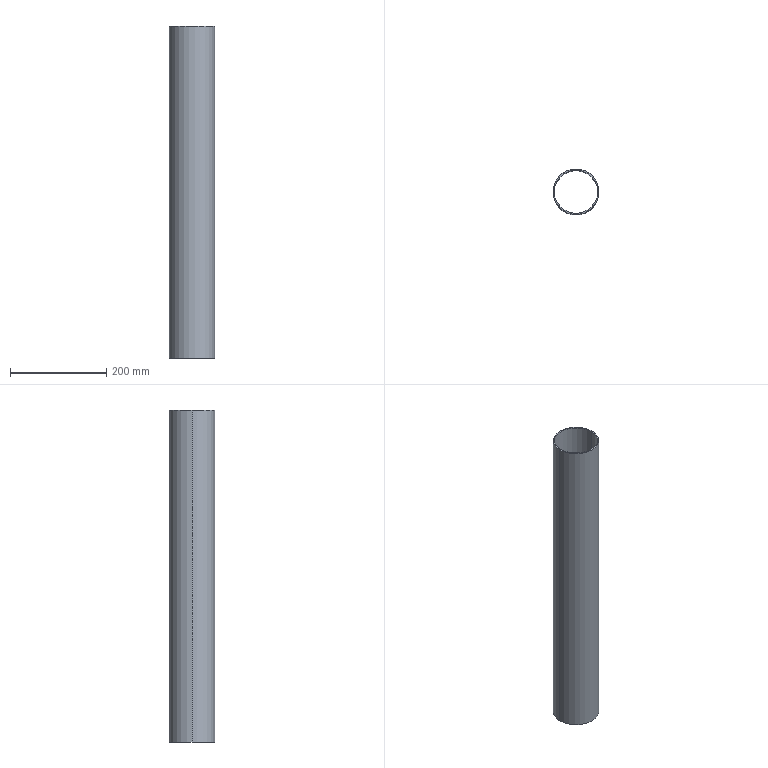Part | SolidWorks | features Extrusion 1 | 1 solid | 6 faces | box 95 x 95 x 690 mm | volume 501280 mm3 | cylinder 4 | plane 2 | commonest cylinder face diameters 90 x2 95 x2
STEP:
#1=CARTESIAN_POINT('',(-45.,0.,345.));
#2=VERTEX_POINT('',#1);
#3=CARTESIAN_POINT('',(45.,0.,345.));
#4=VERTEX_POINT('',#3);
#5=CARTESIAN_POINT('',(0.,0.,345.));
#6=DIRECTION('',(0.,0.,1.));
#7=DIRECTION('',(1.,0.,0.));
#8=AXIS2_PLACEMENT_3D('',#5,#6,#7);
#9=CIRCLE('',#8,45.);
#10=EDGE_CURVE('',#2,#4,#9,.T.);
#11=ORIENTED_EDGE('',*,*,#10,.T.);
#12=CARTESIAN_POINT('',(45.,0.,-345.));
#13=VERTEX_POINT('',#12);
#14=CARTESIAN_POINT('',(45.,0.,345.));
#15=DIRECTION('',(0.,0.,-1.));
#16=VECTOR('',#15,1000.);
#17=LINE('',#14,#16);
#18=EDGE_CURVE('',#4,#13,#17,.T.);
#19=ORIENTED_EDGE('',*,*,#18,.T.);
#20=CARTESIAN_POINT('',(-45.,0.,-345.));
#21=VERTEX_POINT('',#20);
#22=CARTESIAN_POINT('',(0.,0.,-345.));
#23=DIRECTION('',(0.,0.,1.));
#24=DIRECTION('',(1.,0.,0.));
#25=AXIS2_PLACEMENT_3D('',#22,#23,#24);
#26=CIRCLE('',#25,45.);
#27=EDGE_CURVE('',#21,#13,#26,.T.);
#28=ORIENTED_EDGE('',*,*,#27,.F.);
#29=CARTESIAN_POINT('',(-45.,0.,345.));
#30=DIRECTION('',(0.,0.,-1.));
#31=VECTOR('',#30,1000.);
#32=LINE('',#29,#31);
#33=EDGE_CURVE('',#2,#21,#32,.T.);
#34=ORIENTED_EDGE('',*,*,#33,.F.);
#35=EDGE_LOOP('',(#11,#19,#28,#34));
#36=FACE_OUTER_BOUND('',#35,.T.);
#37=CARTESIAN_POINT('',(0.,0.,345.));
#38=DIRECTION('',(0.,0.,-1.));
#39=DIRECTION('',(-1.,0.,0.));
#40=AXIS2_PLACEMENT_3D('',#37,#38,#39);
#41=CYLINDRICAL_SURFACE('',#40,45.);
#42=ADVANCED_FACE('',(#36),#41,.F.);
#43=CARTESIAN_POINT('',(47.5,0.,345.));
#44=VERTEX_POINT('',#43);
#45=CARTESIAN_POINT('',(-47.5,0.,345.));
#46=VERTEX_POINT('',#45);
#47=CARTESIAN_POINT('',(0.,0.,345.));
#48=DIRECTION('',(0.,0.,1.));
#49=DIRECTION('',(1.,0.,0.));
#50=AXIS2_PLACEMENT_3D('',#47,#48,#49);
#51=CIRCLE('',#50,47.5);
#52=EDGE_CURVE('',#44,#46,#51,.T.);
#53=ORIENTED_EDGE('',*,*,#52,.F.);
#54=CARTESIAN_POINT('',(47.5,0.,-345.));
#55=VERTEX_POINT('',#54);
#56=CARTESIAN_POINT('',(47.5,0.,345.));
#57=DIRECTION('',(0.,0.,-1.));
#58=VECTOR('',#57,1000.);
#59=LINE('',#56,#58);
#60=EDGE_CURVE('',#44,#55,#59,.T.);
#61=ORIENTED_EDGE('',*,*,#60,.T.);
#62=CARTESIAN_POINT('',(-47.5,0.,-345.));
#63=VERTEX_POINT('',#62);
#64=CARTESIAN_POINT('',(0.,0.,-345.));
#65=DIRECTION('',(0.,0.,1.));
#66=DIRECTION('',(1.,0.,0.));
#67=AXIS2_PLACEMENT_3D('',#64,#65,#66);
#68=CIRCLE('',#67,47.5);
#69=EDGE_CURVE('',#55,#63,#68,.T.);
#70=ORIENTED_EDGE('',*,*,#69,.T.);
#71=CARTESIAN_POINT('',(-47.5,0.,345.));
#72=DIRECTION('',(0.,0.,-1.));
#73=VECTOR('',#72,1000.);
#74=LINE('',#71,#73);
#75=EDGE_CURVE('',#46,#63,#74,.T.);
#76=ORIENTED_EDGE('',*,*,#75,.F.);
#77=EDGE_LOOP('',(#53,#61,#70,#76));
#78=FACE_OUTER_BOUND('',#77,.T.);
#79=CARTESIAN_POINT('',(0.,0.,345.));
#80=DIRECTION('',(0.,0.,-1.));
#81=DIRECTION('',(-1.,0.,0.));
#82=AXIS2_PLACEMENT_3D('',#79,#80,#81);
#83=CYLINDRICAL_SURFACE('',#82,47.5);
#84=ADVANCED_FACE('',(#78),#83,.T.);
#85=CARTESIAN_POINT('',(0.,0.,345.));
#86=DIRECTION('',(0.,0.,1.));
#87=DIRECTION('',(1.,0.,0.));
#88=AXIS2_PLACEMENT_3D('',#85,#86,#87);
#89=CIRCLE('',#88,47.5);
#90=EDGE_CURVE('',#46,#44,#89,.T.);
#91=ORIENTED_EDGE('',*,*,#90,.T.);
#92=ORIENTED_EDGE('',*,*,#52,.T.);
#93=EDGE_LOOP('',(#91,#92));
#94=FACE_OUTER_BOUND('',#93,.T.);
#95=ORIENTED_EDGE('',*,*,#10,.F.);
#96=CARTESIAN_POINT('',(0.,0.,345.));
#97=DIRECTION('',(0.,0.,1.));
#98=DIRECTION('',(1.,0.,0.));
#99=AXIS2_PLACEMENT_3D('',#96,#97,#98);
#100=CIRCLE('',#99,45.);
#101=EDGE_CURVE('',#4,#2,#100,.T.);
#102=ORIENTED_EDGE('',*,*,#101,.F.);
#103=EDGE_LOOP('',(#95,#102));
#104=FACE_BOUND('',#103,.T.);
#105=CARTESIAN_POINT('',(0.,0.,345.));
#106=DIRECTION('',(0.,0.,1.));
#107=DIRECTION('',(1.,0.,0.));
#108=AXIS2_PLACEMENT_3D('',#105,#106,#107);
#109=PLANE('',#108);
#110=ADVANCED_FACE('',(#94,#104),#109,.T.);
#111=CARTESIAN_POINT('',(0.,0.,-345.));
#112=DIRECTION('',(0.,0.,1.));
#113=DIRECTION('',(1.,0.,0.));
#114=AXIS2_PLACEMENT_3D('',#111,#112,#113);
#115=CIRCLE('',#114,47.5);
#116=EDGE_CURVE('',#63,#55,#115,.T.);
#117=ORIENTED_EDGE('',*,*,#116,.F.);
#118=ORIENTED_EDGE('',*,*,#69,.F.);
#119=EDGE_LOOP('',(#117,#118));
#120=FACE_OUTER_BOUND('',#119,.T.);
#121=ORIENTED_EDGE('',*,*,#27,.T.);
#122=CARTESIAN_POINT('',(0.,0.,-345.));
#123=DIRECTION('',(0.,0.,1.));
#124=DIRECTION('',(1.,0.,0.));
#125=AXIS2_PLACEMENT_3D('',#122,#123,#124);
#126=CIRCLE('',#125,45.);
#127=EDGE_CURVE('',#13,#21,#126,.T.);
#128=ORIENTED_EDGE('',*,*,#127,.T.);
#129=EDGE_LOOP('',(#121,#128));
#130=FACE_BOUND('',#129,.T.);
#131=CARTESIAN_POINT('',(0.,0.,-345.));
#132=DIRECTION('',(0.,0.,1.));
#133=DIRECTION('',(1.,0.,0.));
#134=AXIS2_PLACEMENT_3D('',#131,#132,#133);
#135=PLANE('',#134);
#136=ADVANCED_FACE('',(#120,#130),#135,.F.);
#137=ORIENTED_EDGE('',*,*,#60,.F.);
#138=ORIENTED_EDGE('',*,*,#90,.F.);
#139=ORIENTED_EDGE('',*,*,#75,.T.);
#140=ORIENTED_EDGE('',*,*,#116,.T.);
#141=EDGE_LOOP('',(#137,#138,#139,#140));
#142=FACE_OUTER_BOUND('',#141,.T.);
#143=CARTESIAN_POINT('',(0.,0.,345.));
#144=DIRECTION('',(0.,0.,-1.));
#145=DIRECTION('',(-1.,0.,0.));
#146=AXIS2_PLACEMENT_3D('',#143,#144,#145);
#147=CYLINDRICAL_SURFACE('',#146,47.5);
#148=ADVANCED_FACE('',(#142),#147,.T.);
#149=ORIENTED_EDGE('',*,*,#18,.F.);
#150=ORIENTED_EDGE('',*,*,#101,.T.);
#151=ORIENTED_EDGE('',*,*,#33,.T.);
#152=ORIENTED_EDGE('',*,*,#127,.F.);
#153=EDGE_LOOP('',(#149,#150,#151,#152));
#154=FACE_OUTER_BOUND('',#153,.T.);
#155=CARTESIAN_POINT('',(0.,0.,345.));
#156=DIRECTION('',(0.,0.,-1.));
#157=DIRECTION('',(-1.,0.,0.));
#158=AXIS2_PLACEMENT_3D('',#155,#156,#157);
#159=CYLINDRICAL_SURFACE('',#158,45.);
#160=ADVANCED_FACE('',(#154),#159,.F.);
#161=CLOSED_SHELL('',(#42,#84,#110,#136,#148,#160));
#162=MANIFOLD_SOLID_BREP('',#161);
#163=CARTESIAN_POINT('',(0.,0.,0.));
#164=DIRECTION('',(0.,0.,1.));
#165=DIRECTION('',(1.,0.,0.));
#166=AXIS2_PLACEMENT_3D('',#163,#164,#165);
#167=(LENGTH_UNIT()NAMED_UNIT(*)SI_UNIT(.MILLI.,.METRE.));
#168=UNCERTAINTY_MEASURE_WITH_UNIT(LENGTH_MEASURE(0.00001),#167,'','');
#169=(NAMED_UNIT(*)PLANE_ANGLE_UNIT()SI_UNIT($,.RADIAN.));
#170=(NAMED_UNIT(*)SI_UNIT($,.STERADIAN.)SOLID_ANGLE_UNIT());
#171=(GEOMETRIC_REPRESENTATION_CONTEXT(3)GLOBAL_UNCERTAINTY_ASSIGNED_CONTEXT((#168))GLOBAL_UNIT_ASSIGNED_CONTEXT((#167,#169,#170))REPRESENTATION_CONTEXT('',''));
#172=ADVANCED_BREP_SHAPE_REPRESENTATION('',(#162,#166),#171);